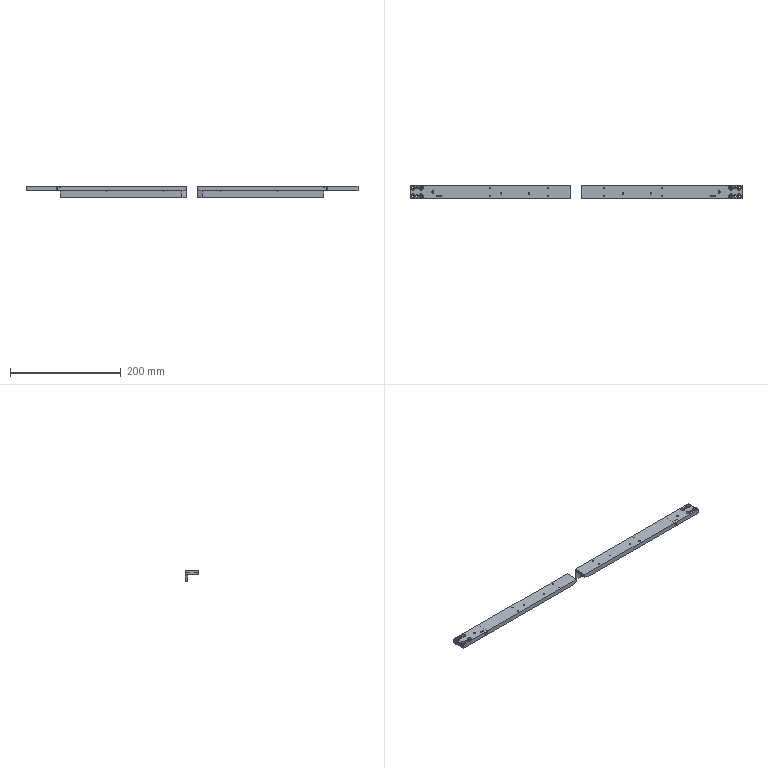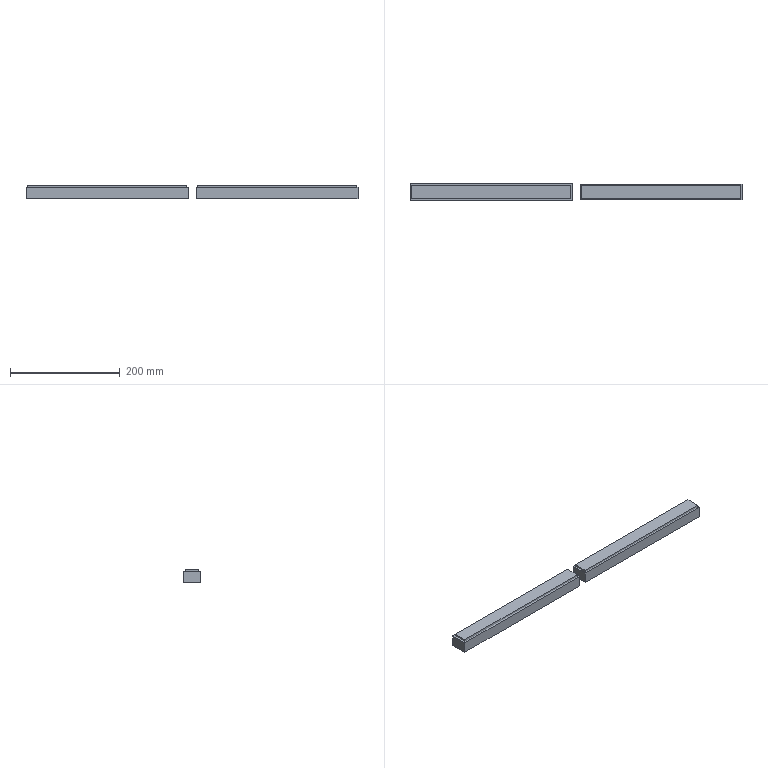CAM job | NX | 3-axis milling, drilling | part box 600 x 25 x 20 mm | stock box 605 x 31 x 25 mm
Tools:
number,name,description,diameter,corner_radius,flute_length,length,flutes
1,D50,Milling Tool-5 Parameters,50.0,0.0,50.0,75.0,2
2,D6A45,Milling Tool-5 Parameters,6.0,0.0,3.0,3.0,2
14,4.5ZT,Drilling Tool,4.5,0.0,35.0,50.0,2
12,2.5ZT,Drilling Tool,2.5,0.0,35.0,50.0,2
3,D10,Milling Tool-5 Parameters,10.0,0.0,50.0,75.0,2
8,D6,Milling Tool-5 Parameters,6.0,0.0,50.0,75.0,2
20,D3,Milling Tool-5 Parameters,3.0,0.0,50.0,75.0,2
13,4.2ZT,Drilling Tool,4.2,0.0,35.0,50.0,2
4,D10JING,Milling Tool-5 Parameters,10.0,0.0,50.0,75.0,2
20,D6R0.5,Milling Tool-5 Parameters,6.0,0.5,50.0,75.0,2
Operations:
program,operation,operation_type,tool,method,geometry_group,spindle_rpm,surface_speed,feed_per_tooth,feed_cut,feed_plunge,cut_length_mm,path_length_mm,cut_time_min,machine_time_min
1-293-25-25毛胚-虎钳,FLOOR_WALL,VolumeBased25DMillingOperation,D50,METHOD,A,6500.0,1286.0,0.0962,1250.0,100.0,358.0,412.0,0.2864,0.2918
1-293-25-25毛胚-虎钳,DRILLING_COPY_1,Operation,D6A45,METHOD,A,3000.0,56.0,0.0333,200.0,0.0,69.0,555.367,0.345,0.3936
1-293-25-25毛胚-虎钳,DRILLING_COPY_1_COPY_COPY_1_COPY_1_COPY,Operation,4.5ZT,METHOD,A,2000.0,18.0,0.03,120.0,0.0,55.408,225.707,0.4617,0.4788
1-293-25-25毛胚-虎钳,DRILLING_COPY_1_COPY_COPY_1_COPY_1_COPY_COPY_1,Operation,4.2ZT,METHOD,A,2000.0,18.0,0.03,120.0,0.0,13.762,87.524,0.1147,0.1221
1-293-25-25毛胚-虎钳,DRILLING_COPY_1_COPY_COPY_1_COPY_1_COPY_COPY,Operation,2.5ZT,METHOD,A,2000.0,18.0,0.03,120.0,0.0,124.511,621.587,1.038,1.087
1-293-25-25毛胚-虎钳,ZLEVEL_PROFILE,ZLevelMilling,D10,METHOD,A,7000.0,219.0,0.2143,3000.0,1000.0,13347.609,13424.609,4.481,4.489
1-293-25-25毛胚-虎钳,ZLEVEL_PROFILE_COPY_COPY_1_COPY_COPY_COPY_1,ZLevelMilling,D10JING,METHOD,A,7000.0,219.0,0.0714,1000.0,100.0,664.548,764.548,0.6645,0.6745
1-293-25-25毛胚-虎钳,HOLE_MILLING_1,CylinderMilling,D6,METHOD,A,7000.0,131.0,0.1071,1500.0,100.0,284.779,585.379,0.1899,0.2199
1-293-25-25毛胚-虎钳,ZLEVEL_PROFILE_COPY_1_COPY,ZLevelMilling,D3,METHOD,A,7000.0,65.0,0.0929,1300.0,1000.0,263.194,410.602,0.2139,0.2286
1-293-25-25毛胚-虎钳,ZLEVEL_PROFILE_COPY_1_COPY_COPY_COPY_COPY_2_COPY,ZLevelMilling,D6A45,METHOD,A,7000.0,131.0,0.0714,1000.0,1000.0,787.575,2823.402,0.7876,0.9912
1-293-25-25毛胚-虎钳,刀补10_COPY,ZLevelMilling,D3,METHOD,A,7000.0,87.0,0.0607,850.0,1000.0,73.319,223.961,0.0859,0.1009
2-293-25-25毛胚-虎钳,FLOOR_WALL_COPY,VolumeBased25DMillingOperation,D50,METHOD,B,6500.0,1286.0,0.0962,1250.0,100.0,1760.0,3394.001,1.408,1.571
2-293-25-25毛胚-虎钳,FLOOR_WALL_1,VolumeBased25DMillingOperation,D10,METHOD,B,7000.0,219.0,0.2143,3000.0,1000.0,7177.99,7892.595,2.415,2.486
2-293-25-25毛胚-虎钳,FLOOR_WALL_1_COPY_1,VolumeBased25DMillingOperation,D10JING,METHOD,B,7000.0,87.0,0.0714,1000.0,100.0,1694.058,1850.539,1.694,1.714
2-293-25-25毛胚-虎钳,ZLEVEL_PROFILE_COPY_COPY_1_COPY_COPY_COPY_1_COPY_COPY,ZLevelMilling,D6R0.5,METHOD,B,7000.0,131.0,0.2143,3000.0,1000.0,1870.454,1957.669,0.6241,0.6328
2-293-25-25毛胚-虎钳,ZLEVEL_PROFILE_COPY_1_COPY_COPY_COPY_COPY_2_COPY_COPY,ZLevelMilling,D6A45,METHOD,B,7000.0,131.0,0.0714,1000.0,1000.0,471.073,533.073,0.4711,0.4773
2-293-25-25毛胚-虎钳,ZLEVEL_PROFILE_COPY_1_COPY_COPY_COPY_COPY_2_COPY_COPY_COPY,ZLevelMilling,D6A45,METHOD,B,7000.0,131.0,0.0714,1000.0,1000.0,458.948,2129.532,0.4589,0.626
1对称-293-25-25毛胚-虎钳,FLOOR_WALL_2,VolumeBased25DMillingOperation,D50,METHOD,A,6500.0,1286.0,0.0962,1250.0,100.0,358.0,412.0,0.2864,0.2918
1对称-293-25-25毛胚-虎钳,DRILLING_COPY_1_1,Operation,D6A45,METHOD,A,3000.0,56.0,0.0333,200.0,0.0,69.0,555.367,0.345,0.3936
1对称-293-25-25毛胚-虎钳,DRILLING_COPY_1_COPY_COPY_1_COPY_1_COPY_1,Operation,4.5ZT,METHOD,A,2000.0,18.0,0.03,120.0,0.0,55.408,225.707,0.4617,0.4788
1对称-293-25-25毛胚-虎钳,DRILLING_COPY_1_COPY_COPY_1_COPY_1_COPY_COPY_1_1,Operation,4.2ZT,METHOD,A,2000.0,18.0,0.03,120.0,0.0,13.762,87.524,0.1147,0.1221
1对称-293-25-25毛胚-虎钳,DRILLING_COPY_1_COPY_COPY_1_COPY_1_COPY_COPY_2,Operation,2.5ZT,METHOD,A,2000.0,18.0,0.03,120.0,0.0,124.511,621.587,1.038,1.087
1对称-293-25-25毛胚-虎钳,ZLEVEL_PROFILE_1,ZLevelMilling,D10,METHOD,A,7000.0,219.0,0.2143,3000.0,1000.0,13347.609,13424.609,4.481,4.489
1对称-293-25-25毛胚-虎钳,ZLEVEL_PROFILE_COPY_COPY_1_COPY_COPY_COPY_1_1,ZLevelMilling,D10JING,METHOD,A,7000.0,219.0,0.0714,1000.0,100.0,664.548,764.548,0.6645,0.6745
1对称-293-25-25毛胚-虎钳,HOLE_MILLING_1_1,CylinderMilling,D6,METHOD,A,7000.0,131.0,0.1071,1500.0,100.0,284.779,585.379,0.1899,0.2199
1对称-293-25-25毛胚-虎钳,ZLEVEL_PROFILE_COPY_1_COPY_1,ZLevelMilling,D3,METHOD,A,7000.0,65.0,0.0929,1300.0,1000.0,263.323,409.943,0.214,0.2286
1对称-293-25-25毛胚-虎钳,ZLEVEL_PROFILE_COPY_1_COPY_COPY_COPY_COPY_2_COPY_1,ZLevelMilling,D6A45,METHOD,A,7000.0,131.0,0.0714,1000.0,1000.0,787.575,3021.348,0.7876,1.011
1对称-293-25-25毛胚-虎钳,刀补10_COPY_1,ZLevelMilling,D3,METHOD,A,7000.0,87.0,0.0607,850.0,1000.0,73.341,224.571,0.0859,0.101
2对称-293-25-25毛胚-虎钳,FLOOR_WALL_COPY_1,VolumeBased25DMillingOperation,D50,METHOD,B,6500.0,1286.0,0.0962,1250.0,100.0,1760.0,3394.001,1.408,1.571
2对称-293-25-25毛胚-虎钳,FLOOR_WALL_1_1,VolumeBased25DMillingOperation,D10,METHOD,B,7000.0,219.0,0.2143,3000.0,1000.0,7165.909,7971.478,2.412,2.493
2对称-293-25-25毛胚-虎钳,FLOOR_WALL_1_COPY_1_1,VolumeBased25DMillingOperation,D10JING,METHOD,B,7000.0,87.0,0.0714,1000.0,100.0,2232.041,2409.685,2.232,2.25
2对称-293-25-25毛胚-虎钳,ZLEVEL_PROFILE_COPY_COPY_1_COPY_COPY_COPY_1_COPY_COPY_1,ZLevelMilling,D6R0.5,METHOD,B,7000.0,131.0,0.2143,3000.0,1000.0,1870.454,1957.669,0.6241,0.6328
2对称-293-25-25毛胚-虎钳,ZLEVEL_PROFILE_COPY_1_COPY_COPY_COPY_COPY_2_COPY_COPY_1,ZLevelMilling,D6A45,METHOD,B,7000.0,131.0,0.0714,1000.0,1000.0,471.087,533.087,0.4711,0.4773
2对称-293-25-25毛胚-虎钳,ZLEVEL_PROFILE_COPY_1_COPY_COPY_COPY_COPY_2_COPY_COPY_COPY_1,ZLevelMilling,D6A45,METHOD,B,7000.0,131.0,0.0714,1000.0,1000.0,458.948,2354.15,0.4589,0.6485